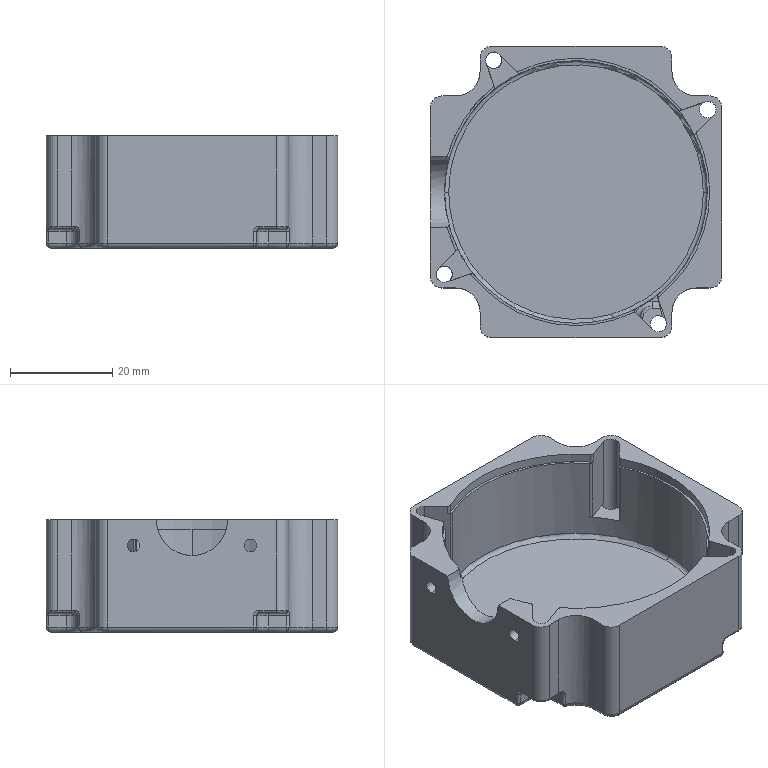Part | NX | features BREP 1 | 1 solid | 191 faces | box 57.15 x 57.15 x 22 mm | volume 19756 mm3 | cylinder 102 | plane 45 | torus 30 | spline 12 | cone 2 | commonest cylinder face diameters 1 x45 2 x16 4.6 x12 3.2 x11 52.4 x5 2.5 x4